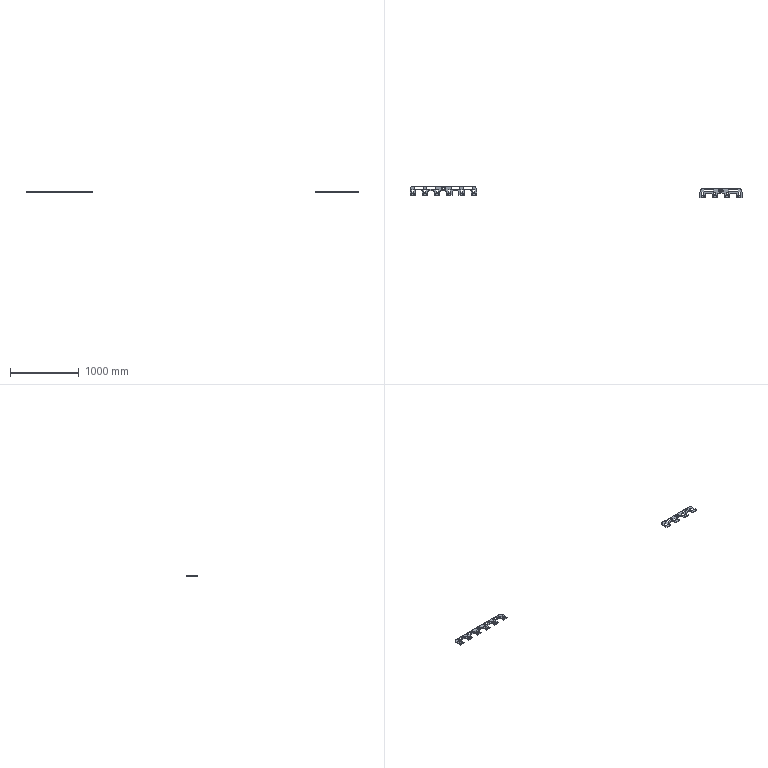NC program | NX | posted with a generic post | part box 4825 x 168.213 x 13 mm
Lines 1 to 1365 of 4378:
N10 G17 G21 G94 G90
(FLOOR_WALL_COPY_COPY , TOOL : D63)
N12 T01 M6
N14 G54
N16 G17 G0 G90 X519.9 Y-101.997 S6500 M3
N18 G43 Z30. H1
N20 Z4.
N22 G94 G1 Z1. F1500.
N24 X516.9
N26 X107.8
N28 Y-73.798
N30 X516.9
N32 Y-45.599
N34 X107.8
N36 Y-17.399
N38 X516.9
N40 Y10.8
N42 X107.8
N44 Y38.999
N46 X516.9
N48 X519.9
N50 Z4.
N52 G0 Z30.
N54 Y-101.997
N56 Z3.
N58 G1 Z0.
N60 X516.9
N62 X107.8
N64 Y-73.798
N66 X516.9
N68 Y-45.599
N70 X107.8
N72 Y-17.399
N74 X516.9
N76 Y10.8
N78 X107.8
N80 Y38.999
N82 X516.9
N84 X519.9
N86 Z3.
N88 G0 Z30.
N90 M5
(DRILLING_COPY_1_COPY , TOOL : D6A45)
N92 T07 M6
N94 G54
N96 G17 G0 G90 X464.5 Y-72.2 S5000 M3
N98 G43 Z30. H7
N100 G94 G81 G98 Z-1. F250. R3.
N102 Y-94.2
N104 X424.5
N106 Y-72.2
N108 X286.7
N110 Y-94.2
N112 X246.7
N114 Y-72.2
N116 G80
N118 G0 X246.7 Y-72.2 Z30.
N120 M5
(DRILLING_COPY_COPY_COPY_COPY , TOOL : 6.5ZT)
N122 T15 M6
N124 G54
N126 G17 G0 G90 X464.5 Y-72.2 S2000 M3
N128 G43 Z30. H15
N130 G94 G83 G98 Z-15.953 F250. Q2. R3.
N132 Y-94.2
N134 X424.5
N136 Y-72.2
N138 X286.7
N140 Y-94.2
N142 X246.7
N144 Y-72.2
N146 G80
N148 G0 X246.7 Y-72.2 Z30.
N150 M5
(ZLEVEL_PROFILE_COPY_3_COPY_1 , TOOL : D10)
N152 T10 M6
N154 G54
N156 G17 G0 G90 X105.202 Y42.6 S9500 M3
N158 G43 Z30. H10
N160 Z4.
N162 G94 G1 Z-1. F1000.
N164 X106.934 Y39.6
N166 G3 X107.8 Y39.1 R1.
N168 G1 X433.4 F3500.
N170 G2 X488.5 Y-16. R55.1
N172 G1 Y-100.
N174 G2 X483.4 Y-105.1 R5.1
N176 G1 X405.6
N178 G2 X400.5 Y-100. R5.1
N180 G1 Y-38.
N182 G3 X385.6 Y-23.1 R14.9
N184 G1 X325.6
N186 G3 X310.7 Y-38. R14.9
N188 G1 Y-100.
N190 G2 X305.6 Y-105.1 R5.1
N192 G1 X227.8
N194 G2 X222.7 Y-100. R5.1
N196 G1 Y-53.95
N198 G3 X207.8 Y-39.05 R14.9
N200 G1 X147.8
N202 G3 X132.9 Y-53.95 R14.9
N204 G1 Y-100.
N206 G2 X127.8 Y-105.1 R5.1
N208 G1 X107.8
N210 G3 X106.934 Y-105.6 R1.
N212 G1 X105.202 Y-108.6
N214 Z4.
N216 G0 Z30.
N218 Z3.
N220 G1 Z-2. F1000.
N222 X106.934 Y-105.6
N224 G2 X107.8 Y-105.1 R1.
N226 G1 X127.8 F3500.
N228 G3 X132.9 Y-100. R5.1
N230 G1 Y-53.95
N232 G2 X147.8 Y-39.05 R14.9
N234 G1 X207.8
N236 G2 X222.7 Y-53.95 R14.9
N238 G1 Y-100.
N240 G3 X227.8 Y-105.1 R5.1
N242 G1 X305.6
N244 G3 X310.7 Y-100. R5.1
N246 G1 Y-38.
N248 G2 X325.6 Y-23.1 R14.9
N250 G1 X385.6
N252 G2 X400.5 Y-38. R14.9
N254 G1 Y-100.
N256 G3 X405.6 Y-105.1 R5.1
N258 G1 X483.4
N260 G3 X488.5 Y-100. R5.1
N262 G1 Y-16.
N264 G3 X433.4 Y39.1 R55.1
N266 G1 X107.8
N268 G2 X106.934 Y39.6 R1.
N270 G1 X105.202 Y42.6
N272 Z3.
N274 G0 Z30.
N276 Z2.
N278 G1 Z-3. F1000.
N280 X106.934 Y39.6
N282 G3 X107.8 Y39.1 R1.
N284 G1 X433.4 F3500.
N286 G2 X488.5 Y-16. R55.1
N288 G1 Y-100.
N290 G2 X483.4 Y-105.1 R5.1
N292 G1 X405.6
N294 G2 X400.5 Y-100. R5.1
N296 G1 Y-38.
N298 G3 X385.6 Y-23.1 R14.9
N300 G1 X325.6
N302 G3 X310.7 Y-38. R14.9
N304 G1 Y-100.
N306 G2 X305.6 Y-105.1 R5.1
N308 G1 X227.8
N310 G2 X222.7 Y-100. R5.1
N312 G1 Y-53.95
N314 G3 X207.8 Y-39.05 R14.9
N316 G1 X147.8
N318 G3 X132.9 Y-53.95 R14.9
N320 G1 Y-100.
N322 G2 X127.8 Y-105.1 R5.1
N324 G1 X107.8
N326 G3 X106.934 Y-105.6 R1.
N328 G1 X105.202 Y-108.6
N330 Z2.
N332 G0 Z30.
N334 Z1.2
N336 G1 Z-3.8 F1000.
N338 X106.934 Y-105.6
N340 G2 X107.8 Y-105.1 R1.
N342 G1 X127.8 F3500.
N344 G3 X132.9 Y-100. R5.1
N346 G1 Y-53.95
N348 G2 X147.8 Y-39.05 R14.9
N350 G1 X207.8
N352 G2 X222.7 Y-53.95 R14.9
N354 G1 Y-100.
N356 G3 X227.8 Y-105.1 R5.1
N358 G1 X305.6
N360 G3 X310.7 Y-100. R5.1
N362 G1 Y-38.
N364 G2 X325.6 Y-23.1 R14.9
N366 G1 X385.6
N368 G2 X400.5 Y-38. R14.9
N370 G1 Y-100.
N372 G3 X405.6 Y-105.1 R5.1
N374 G1 X483.4
N376 G3 X488.5 Y-100. R5.1
N378 G1 Y-16.
N380 G3 X433.4 Y39.1 R55.1
N382 G1 X107.8
N384 G2 X106.934 Y39.6 R1.
N386 G1 X105.202 Y42.6
N388 Z1.2
N390 G0 Z30.
N392 Z0.4
N394 G1 Z-4.6 F1000.
N396 X106.934 Y39.6
N398 G3 X107.8 Y39.1 R1.
N400 G1 X433.4 F3500.
N402 G2 X488.5 Y-16. R55.1
N404 G1 Y-100.
N406 G2 X483.4 Y-105.1 R5.1
N408 G1 X405.6
N410 G2 X400.5 Y-100. R5.1
N412 G1 Y-38.
N414 G3 X385.6 Y-23.1 R14.9
N416 G1 X325.6
N418 G3 X310.7 Y-38. R14.9
N420 G1 Y-100.
N422 G2 X305.6 Y-105.1 R5.1
N424 G1 X227.8
N426 G2 X222.7 Y-100. R5.1
N428 G1 Y-53.95
N430 G3 X207.8 Y-39.05 R14.9
N432 G1 X147.8
N434 G3 X132.9 Y-53.95 R14.9
N436 G1 Y-100.
N438 G2 X127.8 Y-105.1 R5.1
N440 G1 X107.8
N442 G3 X106.934 Y-105.6 R1.
N444 G1 X105.202 Y-108.6
N446 Z0.4
N448 G0 Z30.
N450 Z-0.575
N452 G1 Z-5.575 F1000.
N454 X106.934 Y-105.6
N456 G2 X107.8 Y-105.1 R1.
N458 G1 X127.8 F3500.
N460 G3 X132.9 Y-100. R5.1
N462 G1 Y-53.95
N464 G2 X147.8 Y-39.05 R14.9
N466 G1 X207.8
N468 G2 X222.7 Y-53.95 R14.9
N470 G1 Y-100.
N472 G3 X227.8 Y-105.1 R5.1
N474 G1 X305.6
N476 G3 X310.7 Y-100. R5.1
N478 G1 Y-38.
N480 G2 X325.6 Y-23.1 R14.9
N482 G1 X385.6
N484 G2 X400.5 Y-38. R14.9
N486 G1 Y-100.
N488 G3 X405.6 Y-105.1 R5.1
N490 G1 X483.4
N492 G3 X488.5 Y-100. R5.1
N494 G1 Y-16.
N496 G3 X433.4 Y39.1 R55.1
N498 G1 X107.8
N500 G2 X106.934 Y39.6 R1.
N502 G1 X105.202 Y42.6
N504 Z-0.575
N506 G0 Z30.
N508 Z-1.55
N510 G1 Z-6.55 F1000.
N512 X106.934 Y39.6
N514 G3 X107.8 Y39.1 R1.
N516 G1 X433.4 F3500.
N518 G2 X488.5 Y-16. R55.1
N520 G1 Y-100.
N522 G2 X483.4 Y-105.1 R5.1
N524 G1 X405.6
N526 G2 X400.5 Y-100. R5.1
N528 G1 Y-38.
N530 G3 X385.6 Y-23.1 R14.9
N532 G1 X325.6
N534 G3 X310.7 Y-38. R14.9
N536 G1 Y-100.
N538 G2 X305.6 Y-105.1 R5.1
N540 G1 X227.8
N542 G2 X222.7 Y-100. R5.1
N544 G1 Y-53.95
N546 G3 X207.8 Y-39.05 R14.9
N548 G1 X147.8
N550 G3 X132.9 Y-53.95 R14.9
N552 G1 Y-100.
N554 G2 X127.8 Y-105.1 R5.1
N556 G1 X107.8
N558 G3 X106.934 Y-105.6 R1.
N560 G1 X105.202 Y-108.6
N562 Z-1.55
N564 G0 Z30.
N566 Z-2.525
N568 G1 Z-7.525 F1000.
N570 X106.934 Y-105.6
N572 G2 X107.8 Y-105.1 R1.
N574 G1 X127.8 F3500.
N576 G3 X132.9 Y-100. R5.1
N578 G1 Y-53.95
N580 G2 X147.8 Y-39.05 R14.9
N582 G1 X207.8
N584 G2 X222.7 Y-53.95 R14.9
N586 G1 Y-100.
N588 G3 X227.8 Y-105.1 R5.1
N590 G1 X305.6
N592 G3 X310.7 Y-100. R5.1
N594 G1 Y-38.
N596 G2 X325.6 Y-23.1 R14.9
N598 G1 X385.6
N600 G2 X400.5 Y-38. R14.9
N602 G1 Y-100.
N604 G3 X405.6 Y-105.1 R5.1
N606 G1 X483.4
N608 G3 X488.5 Y-100. R5.1
N610 G1 Y-16.
N612 G3 X433.4 Y39.1 R55.1
N614 G1 X107.8
N616 G2 X106.934 Y39.6 R1.
N618 G1 X105.202 Y42.6
N620 Z-2.525
N622 G0 Z30.
N624 Z-3.5
N626 G1 Z-8.5 F1000.
N628 X106.934 Y39.6
N630 G3 X107.8 Y39.1 R1.
N632 G1 X433.4 F3500.
N634 G2 X488.5 Y-16. R55.1
N636 G1 Y-100.
N638 G2 X483.4 Y-105.1 R5.1
N640 G1 X405.6
N642 G2 X400.5 Y-100. R5.1
N644 G1 Y-38.
N646 G3 X385.6 Y-23.1 R14.9
N648 G1 X325.6
N650 G3 X310.7 Y-38. R14.9
N652 G1 Y-100.
N654 G2 X305.6 Y-105.1 R5.1
N656 G1 X227.8
N658 G2 X222.7 Y-100. R5.1
N660 G1 Y-53.95
N662 G3 X207.8 Y-39.05 R14.9
N664 G1 X147.8
N666 G3 X132.9 Y-53.95 R14.9
N668 G1 Y-100.
N670 G2 X127.8 Y-105.1 R5.1
N672 G1 X107.8
N674 G3 X106.934 Y-105.6 R1.
N676 G1 X105.202 Y-108.6
N678 Z-3.5
N680 G0 Z30.
N682 Z-4.475
N684 G1 Z-9.475 F1000.
N686 X106.934 Y-105.6
N688 G2 X107.8 Y-105.1 R1.
N690 G1 X127.8 F3500.
N692 G3 X132.9 Y-100. R5.1
N694 G1 Y-53.95
N696 G2 X147.8 Y-39.05 R14.9
N698 G1 X207.8
N700 G2 X222.7 Y-53.95 R14.9
N702 G1 Y-100.
N704 G3 X227.8 Y-105.1 R5.1
N706 G1 X305.6
N708 G3 X310.7 Y-100. R5.1
N710 G1 Y-38.
N712 G2 X325.6 Y-23.1 R14.9
N714 G1 X385.6
N716 G2 X400.5 Y-38. R14.9
N718 G1 Y-100.
N720 G3 X405.6 Y-105.1 R5.1
N722 G1 X483.4
N724 G3 X488.5 Y-100. R5.1
N726 G1 Y-16.
N728 G3 X433.4 Y39.1 R55.1
N730 G1 X107.8
N732 G2 X106.934 Y39.6 R1.
N734 G1 X105.202 Y42.6
N736 Z-4.475
N738 G0 Z30.
N740 Z-5.45
N742 G1 Z-10.45 F1000.
N744 X106.934 Y39.6
N746 G3 X107.8 Y39.1 R1.
N748 G1 X433.4 F3500.
N750 G2 X488.5 Y-16. R55.1
N752 G1 Y-100.
N754 G2 X483.4 Y-105.1 R5.1
N756 G1 X405.6
N758 G2 X400.5 Y-100. R5.1
N760 G1 Y-38.
N762 G3 X385.6 Y-23.1 R14.9
N764 G1 X325.6
N766 G3 X310.7 Y-38. R14.9
N768 G1 Y-100.
N770 G2 X305.6 Y-105.1 R5.1
N772 G1 X227.8
N774 G2 X222.7 Y-100. R5.1
N776 G1 Y-53.95
N778 G3 X207.8 Y-39.05 R14.9
N780 G1 X147.8
N782 G3 X132.9 Y-53.95 R14.9
N784 G1 Y-100.
N786 G2 X127.8 Y-105.1 R5.1
N788 G1 X107.8
N790 G3 X106.934 Y-105.6 R1.
N792 G1 X105.202 Y-108.6
N794 Z-5.45
N796 G0 Z30.
N798 Z-6.425
N800 G1 Z-11.425 F1000.
N802 X106.934 Y-105.6
N804 G2 X107.8 Y-105.1 R1.
N806 G1 X127.8 F3500.
N808 G3 X132.9 Y-100. R5.1
N810 G1 Y-53.95
N812 G2 X147.8 Y-39.05 R14.9
N814 G1 X207.8
N816 G2 X222.7 Y-53.95 R14.9
N818 G1 Y-100.
N820 G3 X227.8 Y-105.1 R5.1
N822 G1 X305.6
N824 G3 X310.7 Y-100. R5.1
N826 G1 Y-38.
N828 G2 X325.6 Y-23.1 R14.9
N830 G1 X385.6
N832 G2 X400.5 Y-38. R14.9
N834 G1 Y-100.
N836 G3 X405.6 Y-105.1 R5.1
N838 G1 X483.4
N840 G3 X488.5 Y-100. R5.1
N842 G1 Y-16.
N844 G3 X433.4 Y39.1 R55.1
N846 G1 X107.8
N848 G2 X106.934 Y39.6 R1.
N850 G1 X105.202 Y42.6
N852 Z-6.425
N854 G0 Z30.
N856 Z-7.4
N858 G1 Z-12.4 F1000.
N860 X106.934 Y39.6
N862 G3 X107.8 Y39.1 R1.
N864 G1 X433.4 F3500.
N866 G2 X488.5 Y-16. R55.1
N868 G1 Y-100.
N870 G2 X483.4 Y-105.1 R5.1
N872 G1 X405.6
N874 G2 X400.5 Y-100. R5.1
N876 G1 Y-38.
N878 G3 X385.6 Y-23.1 R14.9
N880 G1 X325.6
N882 G3 X310.7 Y-38. R14.9
N884 G1 Y-100.
N886 G2 X305.6 Y-105.1 R5.1
N888 G1 X227.8
N890 G2 X222.7 Y-100. R5.1
N892 G1 Y-53.95
N894 G3 X207.8 Y-39.05 R14.9
N896 G1 X147.8
N898 G3 X132.9 Y-53.95 R14.9
N900 G1 Y-100.
N902 G2 X127.8 Y-105.1 R5.1
N904 G1 X107.8
N906 G3 X106.934 Y-105.6 R1.
N908 G1 X105.202 Y-108.6
N910 Z-7.4
N912 G0 Z30.
(ZLEVEL_PROFILE_COPY_2_COPY_COPY , TOOL : D10)
N914 X403.303 Y18.9
N916 Z1.5
N918 G1 X355.6 Z-1. F1000.
N920 X296.835 F3500.
N922 X296.8 Y18.902
N924 Y-2.9
N926 X414.4
N928 Y18.903
N930 X414.348 Y18.9
N932 X355.6
N934 X298.31 Z-2.
N936 X296.835
N938 X296.8 Y18.902
N940 Y-2.9
N942 X414.4
N944 Y18.903
N946 X414.348 Y18.9
N948 X355.6
N950 X298.31 Z-3.
N952 X296.835
N954 X296.8 Y18.902
N956 Y-2.9
N958 X414.4
N960 Y18.903
N962 X414.348 Y18.9
N964 X355.6
N966 X309.768 Z-3.8
N968 X296.835
N970 X296.8 Y18.902
N972 Y-2.9
N974 X414.4
N976 Y18.903
N978 X414.348 Y18.9
N980 X355.6
N982 X309.768 Z-4.6
N984 X296.835
N986 X296.8 Y18.902
N988 Y-2.9
N990 X414.4
N992 Y18.903
N994 X414.348 Y18.9
N996 X355.6
N998 X302.766 Z-5.522
N1000 X296.835
N1002 X296.8 Y18.902
N1004 Y-2.9
N1006 X414.4
N1008 Y18.903
N1010 X414.348 Y18.9
N1012 X355.6
N1014 X302.766 Z-6.444
N1016 X296.835
N1018 X296.8 Y18.902
N1020 Y-2.9
N1022 X414.4
N1024 Y18.903
N1026 X414.348 Y18.9
N1028 X355.6
N1030 X302.766 Z-7.367
N1032 X296.835
N1034 X296.8 Y18.902
N1036 Y-2.9
N1038 X414.4
N1040 Y18.903
N1042 X414.348 Y18.9
N1044 X355.6
N1046 X302.766 Z-8.289
N1048 X296.835
N1050 X296.8 Y18.902
N1052 Y-2.9
N1054 X414.4
N1056 Y18.903
N1058 X414.348 Y18.9
N1060 X355.6
N1062 X302.766 Z-9.211
N1064 X296.835
N1066 X296.8 Y18.902
N1068 Y-2.9
N1070 X414.4
N1072 Y18.903
N1074 X414.348 Y18.9
N1076 X355.6
N1078 X302.766 Z-10.133
N1080 X296.835
N1082 X296.8 Y18.902
N1084 Y-2.9
N1086 X414.4
N1088 Y18.903
N1090 X414.348 Y18.9
N1092 X355.6
N1094 X302.766 Z-11.056
N1096 X296.835
N1098 X296.8 Y18.902
N1100 Y-2.9
N1102 X414.4
N1104 Y18.903
N1106 X414.348 Y18.9
N1108 X355.6
N1110 X302.766 Z-11.978
N1112 X296.835
N1114 X296.8 Y18.902
N1116 Y-2.9
N1118 X414.4
N1120 Y18.903
N1122 X414.348 Y18.9
N1124 X355.6
N1126 X302.766 Z-12.9
N1128 X296.835
N1130 X296.8 Y18.902
N1132 Y-2.9
N1134 X414.4
N1136 Y18.903
N1138 X414.348 Y18.9
N1140 X302.766
N1142 Z-11.4
N1144 G0 Z30.
N1146 X225.503
N1148 Z1.5
N1150 G1 X177.8 Z-1. F1000.
N1152 X119.036 F3500.
N1154 X119. Y18.902
N1156 Y-2.9
N1158 X236.6
N1160 Y18.902
N1162 X236.557 Y18.9
N1164 X177.8
N1166 X120.51 Z-2.
N1168 X119.036
N1170 X119. Y18.902
N1172 Y-2.9
N1174 X236.6
N1176 Y18.902
N1178 X236.557 Y18.9
N1180 X177.8
N1182 X120.51 Z-3.
N1184 X119.036
N1186 X119. Y18.902
N1188 Y-2.9
N1190 X236.6
N1192 Y18.902
N1194 X236.557 Y18.9
N1196 X177.8
N1198 X131.968 Z-3.8
N1200 X119.036
N1202 X119. Y18.902
N1204 Y-2.9
N1206 X236.6
N1208 Y18.902
N1210 X236.557 Y18.9
N1212 X177.8
N1214 X131.968 Z-4.6
N1216 X119.036
N1218 X119. Y18.902
N1220 Y-2.9
N1222 X236.6
N1224 Y18.902
N1226 X236.557 Y18.9
N1228 X177.8
N1230 X124.966 Z-5.522
N1232 X119.036
N1234 X119. Y18.902
N1236 Y-2.9
N1238 X236.6
N1240 Y18.902
N1242 X236.557 Y18.9
N1244 X177.8
N1246 X124.966 Z-6.444
N1248 X119.036
N1250 X119. Y18.902
N1252 Y-2.9
N1254 X236.6
N1256 Y18.902
N1258 X236.557 Y18.9
N1260 X177.8
N1262 X124.966 Z-7.367
N1264 X119.036
N1266 X119. Y18.902
N1268 Y-2.9
N1270 X236.6
N1272 Y18.902
N1274 X236.557 Y18.9
N1276 X177.8
N1278 X124.966 Z-8.289
N1280 X119.036
N1282 X119. Y18.902
N1284 Y-2.9
N1286 X236.6
N1288 Y18.902
N1290 X236.557 Y18.9
N1292 X177.8
N1294 X124.966 Z-9.211
N1296 X119.036
N1298 X119. Y18.902
N1300 Y-2.9
N1302 X236.6
N1304 Y18.902
N1306 X236.557 Y18.9
N1308 X177.8
N1310 X124.966 Z-10.133
N1312 X119.036
N1314 X119. Y18.902
N1316 Y-2.9
N1318 X236.6
N1320 Y18.902
N1322 X236.557 Y18.9
N1324 X177.8
N1326 X124.966 Z-11.056
N1328 X119.036
N1330 X119. Y18.902
N1332 Y-2.9
N1334 X236.6
N1336 Y18.902
N1338 X236.557 Y18.9
N1340 X177.8
N1342 X124.966 Z-11.978
N1344 X119.036
N1346 X119. Y18.902
N1348 Y-2.9
N1350 X236.6
N1352 Y18.902
N1354 X236.557 Y18.9
N1356 X177.8
N1358 X124.966 Z-12.9
N1360 X119.036
N1362 X119. Y18.902
N1364 Y-2.9
N1366 X236.6
N1368 Y18.902
N1370 X236.557 Y18.9
N1372 X124.966
N1374 Z-11.4
N1376 G0 Z30.
N1378 X434.6 Y-38.898
N1380 Z1.5
N1382 G1 Y-51.9 Z0.819 F1000.
N1384 X454.4 Z-0.219
N1386 Y-36.999 Z-1.
N1388 Y-22.098 F3500.
N1390 X454.352 Y-22.1
N1392 X434.646
N1394 X434.6 Y-22.097
N1396 Y-51.9
N1398 X454.4
N1400 Y-36.999
N1402 Y-22.344 Z-1.256
N1404 Y-22.1 Z-1.26
N1406 X454.201 Z-1.264
N1408 X434.66 Z-1.605
N1410 X434.6 Z-1.606
N1412 Y-22.481 Z-1.612
N1414 Y-44.686 Z-2.
N1416 Y-51.9
N1418 X454.4
N1420 Y-36.999
N1422 Y-22.344 Z-2.256
N1424 Y-22.1 Z-2.26
N1426 X454.201 Z-2.264
N1428 X434.66 Z-2.605
N1430 X434.6 Z-2.606
N1432 Y-22.481 Z-2.612
N1434 Y-44.686 Z-3.
N1436 Y-51.9
N1438 X454.4
N1440 Y-36.999
N1442 Y-22.315 Z-3.256
N1444 Y-22.1 Z-3.26
N1446 X454.172 Z-3.264
N1448 X435.038 Z-3.598
N1450 X434.817 Z-3.602
N1452 X434.6 Y-22.104 Z-3.606
N1454 Y-33.228 Z-3.8
N1456 Y-51.9
N1458 X454.4
N1460 Y-36.999
N1462 Y-22.315 Z-4.056
N1464 Y-22.1 Z-4.06
N1466 X454.172 Z-4.064
N1468 X435.038 Z-4.398
N1470 X434.817 Z-4.402
N1472 X434.6 Y-22.104 Z-4.406
N1474 Y-33.228 Z-4.6
N1476 Y-51.9
N1478 X454.4
N1480 Y-36.999
N1482 Y-22.348 Z-4.856
N1484 Y-22.1 Z-4.86
N1486 X454.205 Z-4.863
N1488 X434.67 Z-5.204
N1490 X434.6 Z-5.206
N1492 Y-22.471 Z-5.212
N1494 Y-40.231 Z-5.522
N1496 Y-51.9
N1498 X454.4
N1500 Y-36.999
N1502 Y-22.348 Z-5.778
N1504 Y-22.1 Z-5.782
N1506 X454.205 Z-5.786
N1508 X434.67 Z-6.127
N1510 X434.6 Z-6.128
N1512 Y-22.471 Z-6.134
N1514 Y-40.231 Z-6.444
N1516 Y-51.9
N1518 X454.4
N1520 Y-36.999
N1522 Y-22.348 Z-6.7
N1524 Y-22.1 Z-6.705
N1526 X454.205 Z-6.708
N1528 X434.67 Z-7.049
N1530 X434.6 Z-7.05
N1532 Y-22.471 Z-7.057
N1534 Y-40.231 Z-7.367
N1536 Y-51.9
N1538 X454.4
N1540 Y-36.999
N1542 Y-22.348 Z-7.622
N1544 Y-22.1 Z-7.627
N1546 X454.205 Z-7.63
N1548 X434.67 Z-7.971
N1550 X434.6 Z-7.972
N1552 Y-22.471 Z-7.979
N1554 Y-40.231 Z-8.289
N1556 Y-51.9
N1558 X454.4
N1560 Y-36.999
N1562 Y-22.348 Z-8.545
N1564 Y-22.1 Z-8.549
N1566 X454.205 Z-8.552
N1568 X434.67 Z-8.893
N1570 X434.6 Z-8.895
N1572 Y-22.471 Z-8.901
N1574 Y-40.231 Z-9.211
N1576 Y-51.9
N1578 X454.4
N1580 Y-36.999
N1582 Y-22.348 Z-9.467
N1584 Y-22.1 Z-9.471
N1586 X454.205 Z-9.475
N1588 X434.67 Z-9.816
N1590 X434.6 Z-9.817
N1592 Y-22.471 Z-9.823
N1594 Y-40.231 Z-10.133
N1596 Y-51.9
N1598 X454.4
N1600 Y-36.999
N1602 Y-22.348 Z-10.389
N1604 Y-22.1 Z-10.393
N1606 X454.205 Z-10.397
N1608 X434.67 Z-10.738
N1610 X434.6 Z-10.739
N1612 Y-22.471 Z-10.746
N1614 Y-40.231 Z-11.056
N1616 Y-51.9
N1618 X454.4
N1620 Y-36.999
N1622 Y-22.348 Z-11.311
N1624 Y-22.1 Z-11.316
N1626 X454.205 Z-11.319
N1628 X434.67 Z-11.66
N1630 X434.6 Z-11.661
N1632 Y-22.471 Z-11.668
N1634 Y-40.231 Z-11.978
N1636 Y-51.9
N1638 X454.4
N1640 Y-36.999
N1642 Y-22.348 Z-12.234
N1644 Y-22.1 Z-12.238
N1646 X454.205 Z-12.241
N1648 X434.67 Z-12.582
N1650 X434.6 Z-12.583
N1652 Y-22.471 Z-12.59
N1654 Y-40.231 Z-12.9
N1656 Y-51.9
N1658 X454.4
N1660 Y-22.098
N1662 X454.352 Y-22.1
N1664 X434.646
N1666 X434.6 Y-22.097
N1668 Y-40.231
N1670 Z-11.4
N1672 G0 Z30.
N1674 X256.8 Y-38.897
N1676 Z1.5
N1678 G1 Y-51.9 Z0.819 F1000.
N1680 X276.6 Z-0.219
N1682 Y-37. Z-1.
N1684 Y-22.1 F3500.
N1686 X256.838
N1688 X256.8 Y-22.098
N1690 Y-51.9
N1692 X276.6
N1694 Y-37.
N1696 Y-22.1 Z-1.26
N1698 X256.86 Z-1.605
N1700 X256.8 Z-1.606
N1702 Y-22.482 Z-1.612
N1704 Y-44.688 Z-2.
N1706 Y-51.9
N1708 X276.6
N1710 Y-37.
N1712 Y-22.1 Z-2.26
N1714 X256.86 Z-2.605
N1716 X256.8 Z-2.606
N1718 Y-22.482 Z-2.612
N1720 Y-44.688 Z-3.
N1722 Y-51.9
N1724 X276.6
N1726 Y-37.
N1728 Y-22.1 Z-3.26
N1730 X257.237 Z-3.598
N1732 X257.016 Z-3.602
N1734 X256.8 Y-22.105 Z-3.606
N1736 Y-33.23 Z-3.8
N1738 Y-51.9
N1740 X276.6
N1742 Y-37.
N1744 Y-22.1 Z-4.06
N1746 X257.237 Z-4.398
N1748 X257.016 Z-4.402
N1750 X256.8 Y-22.105 Z-4.406
N1752 Y-33.23 Z-4.6
N1754 Y-51.9
N1756 X276.6
N1758 Y-37.
N1760 Y-22.1 Z-4.86
N1762 X256.869 Z-5.204
N1764 X256.8 Z-5.206
N1766 Y-22.472 Z-5.212
N1768 Y-40.232 Z-5.522
N1770 Y-51.9
N1772 X276.6
N1774 Y-37.
N1776 Y-22.1 Z-5.782
N1778 X256.869 Z-6.127
N1780 X256.8 Z-6.128
N1782 Y-22.472 Z-6.134
N1784 Y-40.232 Z-6.444
N1786 Y-51.9
N1788 X276.6
N1790 Y-37.
N1792 Y-22.1 Z-6.705
N1794 X256.869 Z-7.049
N1796 X256.8 Z-7.05
N1798 Y-22.472 Z-7.057
N1800 Y-40.232 Z-7.367
N1802 Y-51.9
N1804 X276.6
N1806 Y-37.
N1808 Y-22.1 Z-7.627
N1810 X256.869 Z-7.971
N1812 X256.8 Z-7.972
N1814 Y-22.472 Z-7.979
N1816 Y-40.232 Z-8.289
N1818 Y-51.9
N1820 X276.6
N1822 Y-37.
N1824 Y-22.1 Z-8.549
N1826 X256.869 Z-8.893
N1828 X256.8 Z-8.895
N1830 Y-22.472 Z-8.901
N1832 Y-40.232 Z-9.211
N1834 Y-51.9
N1836 X276.6
N1838 Y-37.
N1840 Y-22.1 Z-9.471
N1842 X256.869 Z-9.816
N1844 X256.8 Z-9.817
N1846 Y-22.472 Z-9.823
N1848 Y-40.232 Z-10.133
N1850 Y-51.9
N1852 X276.6
N1854 Y-37.
N1856 Y-22.1 Z-10.393
N1858 X256.869 Z-10.738
N1860 X256.8 Z-10.739
N1862 Y-22.472 Z-10.746
N1864 Y-40.232 Z-11.056
N1866 Y-51.9
N1868 X276.6
N1870 Y-37.
N1872 Y-22.1 Z-11.316
N1874 X256.869 Z-11.66
N1876 X256.8 Z-11.661
N1878 Y-22.472 Z-11.668
N1880 Y-40.232 Z-11.978
N1882 Y-51.9
N1884 X276.6
N1886 Y-37.
N1888 Y-22.1 Z-12.238
N1890 X256.869 Z-12.582
N1892 X256.8 Z-12.583
N1894 Y-22.472 Z-12.59
N1896 Y-40.232 Z-12.9
N1898 Y-51.9
N1900 X276.6
N1902 Y-22.1
N1904 X256.838
N1906 X256.8 Y-22.098
N1908 Y-40.232
N1910 Z-11.4
N1912 G0 Z30.
(ZLEVEL_PROFILE_COPY_COPY_1_COPY , TOOL : D10)
N1914 X434.5 Y-49.315
N1916 Z1.
N1918 G1 Y-52. Z0.527 F1000.
N1920 X454.5 Z-3.
N1922 Y-21.997 F1500.
N1924 X454.453 Y-22.
N1926 X434.534
N1928 X434.5 Y-21.997
N1930 Y-52.
N1932 X454.5
N1934 Y-22.088 Z-3.638
N1936 X454.367 Y-22. Z-3.643
N1938 X434.723 Z-4.062
N1940 X434.5 Y-21.997 Z-4.067
N1942 Y-22.221 Z-4.071
N1944 Y-46.999 Z-4.6
N1946 Y-52.
N1948 X454.5
N1950 Y-22.088 Z-7.91
N1952 X454.367 Y-22. Z-7.935
N1954 X434.723 Z-10.109
N1956 X434.5 Y-21.997 Z-10.133
N1958 Y-22.221 Z-10.158
N1960 Y-46.999 Z-12.9
N1962 Y-52.
N1964 X454.5
N1966 Y-21.997
N1968 X454.453 Y-22.
N1970 X434.534
N1972 X434.5 Y-21.997
N1974 Y-46.999
N1976 Z-11.9
N1978 G0 Z30.
N1980 X236.017 Y-3.
N1982 Z1.
N1984 G1 X236.7 Z0.88 F1000.
N1986 Y19.002 Z-3.
N1988 X236.658 Y19. F1500.
N1990 X118.947
N1992 X118.9 Y19.003
N1994 Y-3.
N1996 X236.7
N1998 Y19.002
N2000 X236.476 Y19. Z-3.004
N2002 X145.036 Z-4.6
N2004 X118.947
N2006 X118.9 Y19.003
N2008 Y-3.
N2010 X236.7
N2012 Y19.002
N2014 X236.477 Y19. Z-4.609
N2016 X119.105 Z-9.254
N2018 X118.9 Y18.984 Z-9.263
N2020 Y-2.925 Z-10.13
N2022 X119.049 Y-3. Z-10.139
N2024 X188.801 Z-12.9
N2026 X236.7
N2028 Y19.002
N2030 X236.658 Y19.
N2032 X118.947
N2034 X118.9 Y19.002
N2036 Y-3.
N2038 X188.801
N2040 Z-11.9
N2042 G0 Z30.
N2044 X413.816
N2046 Z1.
N2048 G1 X414.5 Z0.879 F1000.
N2050 Y19.002 Z-3.
N2052 X414.464 Y19. F1500.
N2054 X296.747
N2056 X296.7 Y19.002
N2058 Y-3.
N2060 X414.5
N2062 Y19.002
N2064 X414.276 Y19. Z-3.004
N2066 X322.836 Z-4.6
N2068 X296.747
N2070 X296.7 Y19.002
N2072 Y-3.
N2074 X414.5
N2076 Y19.002
N2078 X414.276 Y19. Z-4.609
N2080 X296.906 Z-9.254
N2082 X296.7 Y18.984 Z-9.263
N2084 Y-2.925 Z-10.13
N2086 X296.849 Y-3. Z-10.139
N2088 X366.601 Z-12.9
N2090 X414.5
N2092 Y19.002
N2094 X414.464 Y19.
N2096 X296.747
N2098 X296.7 Y19.002
N2100 Y-3.
N2102 X366.601
N2104 Z-11.9
N2106 G0 Z30.
N2108 X256.7 Y-49.315
N2110 Z1.
N2112 G1 Y-52. Z0.527 F1000.
N2114 X276.7 Z-3.
N2116 Y-21.998 F1500.
N2118 X276.654 Y-22.
N2120 X256.743
N2122 X256.7 Y-21.998
N2124 Y-52.
N2126 X276.7
N2128 Y-22.088 Z-3.638
N2130 X276.567 Y-22. Z-3.643
N2132 X256.923 Z-4.062
N2134 X256.7 Y-21.998 Z-4.067
N2136 Y-46.999 Z-4.6
N2138 Y-52.
N2140 X276.7
N2142 Y-22.088 Z-7.91
N2144 X276.566 Y-22. Z-7.935
N2146 X256.923 Z-10.109
N2148 X256.7 Y-21.998 Z-10.133
N2150 Y-46.999 Z-12.9
N2152 Y-52.
N2154 X276.7
N2156 Y-21.999
N2158 X276.654 Y-22.
N2160 X256.743
N2162 X256.7 Y-21.998
N2164 Y-46.999
N2166 Z-11.9
N2168 G0 Z30.
(FLOOR_WALL_1_COPY_1_COPY , TOOL : D10)
N2170 X268.143 Y-106.5
N2172 Z0.533
N2174 G1 Z-0.967 F1000.
N2176 X267.566 Y-105.5
N2178 G3 X266.7 Y-105. R1.
N2180 G1 X222.8 F3000.
N2182 Y-71.5
N2184 X310.6
N2186 Y-105.
N2188 X266.7
N2190 Y-99.
N2192 X228.8
N2194 Y-77.5
N2196 X304.6
N2198 Y-99.
N2200 X266.7
N2202 Y-93.
N2204 X234.8
N2206 Y-83.5
N2208 X298.6
N2210 Y-93.
N2212 X266.7
N2214 Y-88.5
N2216 X239.3
N2218 Y-88.
N2220 X294.1
N2222 Y-88.5
N2224 X266.7
N2226 G3 X265.834 Y-89. R1.
N2228 G1 Z0.533
N2230 G0 X268.143 Y-106.5 Z-0.433
N2232 G1 Z-1.933 F1000.
N2234 X267.566 Y-105.5
N2236 G3 X266.7 Y-105. R1.
N2238 G1 X222.8 F3000.
N2240 Y-71.5
N2242 X310.6
N2244 Y-105.
N2246 X266.7
N2248 Y-99.
N2250 X228.8
N2252 Y-77.5
N2254 X304.6
N2256 Y-99.
N2258 X266.7
N2260 Y-93.
N2262 X234.8
N2264 Y-83.5
N2266 X298.6
N2268 Y-93.
N2270 X266.7
N2272 Y-88.5
N2274 X239.3
N2276 Y-88.
N2278 X294.1
N2280 Y-88.5
N2282 X266.7
N2284 G3 X265.834 Y-89. R1.
N2286 G1 Z-0.433
N2288 G0 X268.143 Y-106.5 Z-1.4
N2290 G1 Z-2.9 F1000.
N2292 X267.566 Y-105.5
N2294 G3 X266.7 Y-105. R1.
N2296 G1 X222.8 F3000.
N2298 Y-71.5
N2300 X310.6
N2302 Y-105.
N2304 X266.7
N2306 Y-99.
N2308 X228.8
N2310 Y-77.5
N2312 X304.6
N2314 Y-99.
N2316 X266.7
N2318 Y-93.
N2320 X234.8
N2322 Y-83.5
N2324 X298.6
N2326 Y-93.
N2328 X266.7
N2330 Y-88.5
N2332 X239.3
N2334 Y-88.
N2336 X294.1
N2338 Y-88.5
N2340 X266.7
N2342 G3 X265.834 Y-89. R1.
N2344 G1 Z-1.4
N2346 G0 Z30.
N2348 X445.943 Y-106.5
N2350 Z0.533
N2352 G1 Z-0.967 F1000.
N2354 X445.366 Y-105.5
N2356 G3 X444.5 Y-105. R1.
N2358 G1 X400.6 F3000.
N2360 Y-71.5
N2362 X488.4
N2364 Y-105.
N2366 X444.5
N2368 Y-99.
N2370 X406.6
N2372 Y-77.5
N2374 X482.4
N2376 Y-99.
N2378 X444.5
N2380 Y-93.
N2382 X412.6
N2384 Y-83.5
N2386 X476.4
N2388 Y-93.
N2390 X444.5
N2392 Y-88.5
N2394 X417.1
N2396 Y-88.
N2398 X471.9
N2400 Y-88.5
N2402 X444.5
N2404 G3 X443.634 Y-89. R1.
N2406 G1 Z0.533
N2408 G0 X445.943 Y-106.5 Z-0.433
N2410 G1 Z-1.933 F1000.
N2412 X445.366 Y-105.5
N2414 G3 X444.5 Y-105. R1.
N2416 G1 X400.6 F3000.
N2418 Y-71.5
N2420 X488.4
N2422 Y-105.
N2424 X444.5
N2426 Y-99.
N2428 X406.6
N2430 Y-77.5
N2432 X482.4
N2434 Y-99.
N2436 X444.5
N2438 Y-93.
N2440 X412.6
N2442 Y-83.5
N2444 X476.4
N2446 Y-93.
N2448 X444.5
N2450 Y-88.5
N2452 X417.1
N2454 Y-88.
N2456 X471.9
N2458 Y-88.5
N2460 X444.5
N2462 G3 X443.634 Y-89. R1.
N2464 G1 Z-0.433
N2466 G0 X445.943 Y-106.5 Z-1.4
N2468 G1 Z-2.9 F1000.
N2470 X445.366 Y-105.5
N2472 G3 X444.5 Y-105. R1.
N2474 G1 X400.6 F3000.
N2476 Y-71.5
N2478 X488.4
N2480 Y-105.
N2482 X444.5
N2484 Y-99.
N2486 X406.6
N2488 Y-77.5
N2490 X482.4
N2492 Y-99.
N2494 X444.5
N2496 Y-93.
N2498 X412.6
N2500 Y-83.5
N2502 X476.4
N2504 Y-93.
N2506 X444.5
N2508 Y-88.5
N2510 X417.1
N2512 Y-88.
N2514 X471.9
N2516 Y-88.5
N2518 X444.5
N2520 G3 X443.634 Y-89. R1.
N2522 G1 Z-1.4
N2524 G0 Z30.
(FLOOR_WALL_1_COPY_COPY_COPY , TOOL : D10)
N2526 X227.303 Y-105.866
N2528 Z-1.5
N2530 G1 Z-3. F1000.
N2532 G3 X227.803 Y-105. R1.
N2534 G1 Y-71.9 F1500.
N2536 X233.48
N2538 Y-105.
N2540 X239.156
N2542 Y-71.9
N2544 X244.833
N2546 Y-105.
N2548 X250.51
N2550 Y-71.9
N2552 X256.186
N2554 Y-105.
N2556 X261.863
N2558 Y-71.9
N2560 X267.54
N2562 Y-105.
N2564 X273.217
N2566 Y-71.9
N2568 X278.893
N2570 Y-105.
N2572 X284.57
N2574 Y-71.9
N2576 X290.247
N2578 Y-105.
N2580 X295.923
N2582 Y-71.9
N2584 X301.6
N2586 Y-105.
N2588 G2 X301.1 Y-105.866 R1.
N2590 G1 Z-1.5
N2592 G0 X311.466 Y-71.9
N2594 G1 Z-3. F1000.
N2596 G3 X310.6 Y-71.4 R1.
N2598 G1 X222.8 F1500.
N2600 G3 X221.934 Y-71.9 R1.
N2602 G1 Z-1.5
N2604 G0 Z30.
N2606 X405.103 Y-105.866
N2608 Z-1.5
N2610 G1 Z-3. F1000.
N2612 G3 X405.603 Y-105. R1.
N2614 G1 Y-71.9 F1500.
N2616 X411.28
N2618 Y-105.
N2620 X416.956
N2622 Y-71.9
N2624 X422.633
N2626 Y-105.
N2628 X428.31
N2630 Y-71.9
N2632 X433.986
N2634 Y-105.
N2636 X439.663
N2638 Y-71.9
N2640 X445.34
N2642 Y-105.
N2644 X451.017
N2646 Y-71.9
N2648 X456.693
N2650 Y-105.
N2652 X462.37
N2654 Y-71.9
N2656 X468.047
N2658 Y-105.
N2660 X473.723
N2662 Y-71.9
N2664 X479.4
N2666 Y-105.
N2668 G2 X478.9 Y-105.866 R1.
N2670 G1 Z-1.5
N2672 G0 X489.266 Y-71.9
N2674 G1 Z-3. F1000.
N2676 G3 X488.4 Y-71.4 R1.
N2678 G1 X400.6 F1500.
N2680 G3 X399.734 Y-71.9 R1.
N2682 G1 Z-1.5
N2684 G0 Z30.
N2686 M5